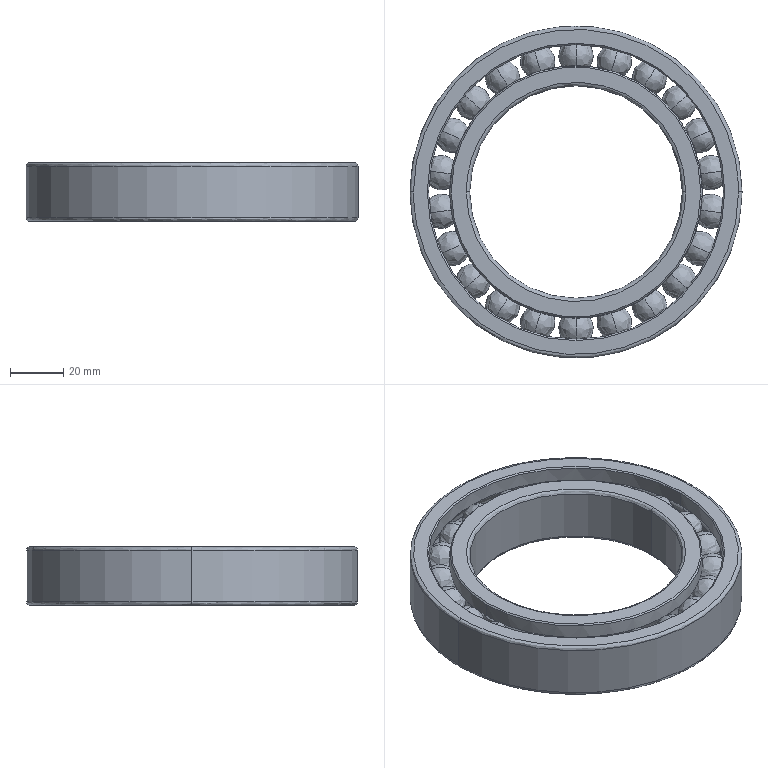Part | STEP file | 7016 | 1 solid | 296 faces | box 125 x 125 x 22 mm | volume 114656 mm3 | spline 186 | plane 90 | cylinder 12 | cone 8 | commonest cylinder face diameters 95 x4 111 x4 80 x2 125 x2